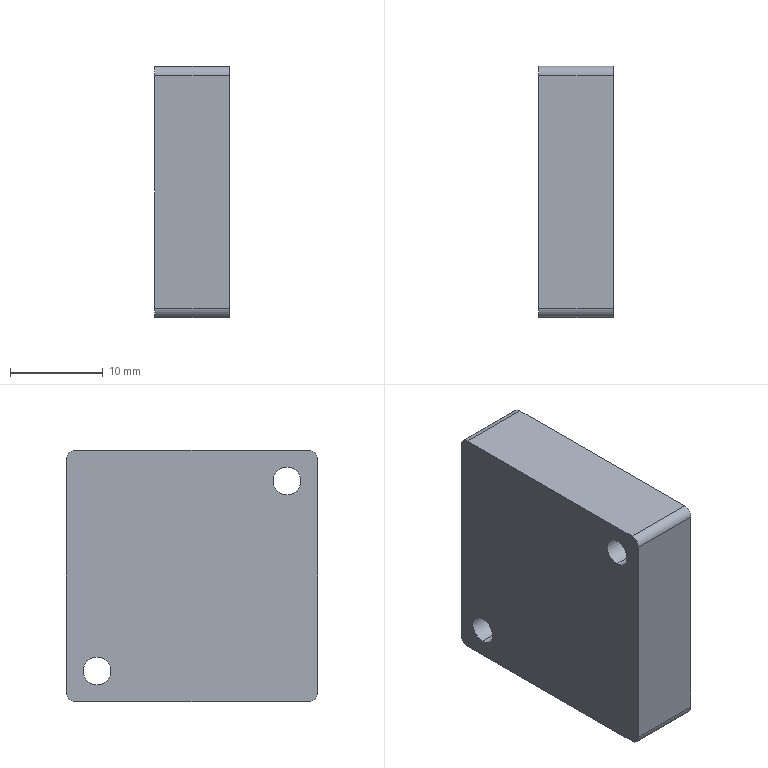Part | SolidWorks | features BaseBody 1 | 1 solid | 182 faces | box 8 x 27.1 x 27.1 mm | volume 5063 mm3 | plane 151 | cylinder 27 | cone 4 | commonest cylinder face diameters 2 x6 3 x6 0.354 x2 0.59 x2 0.8 x2 4 x2